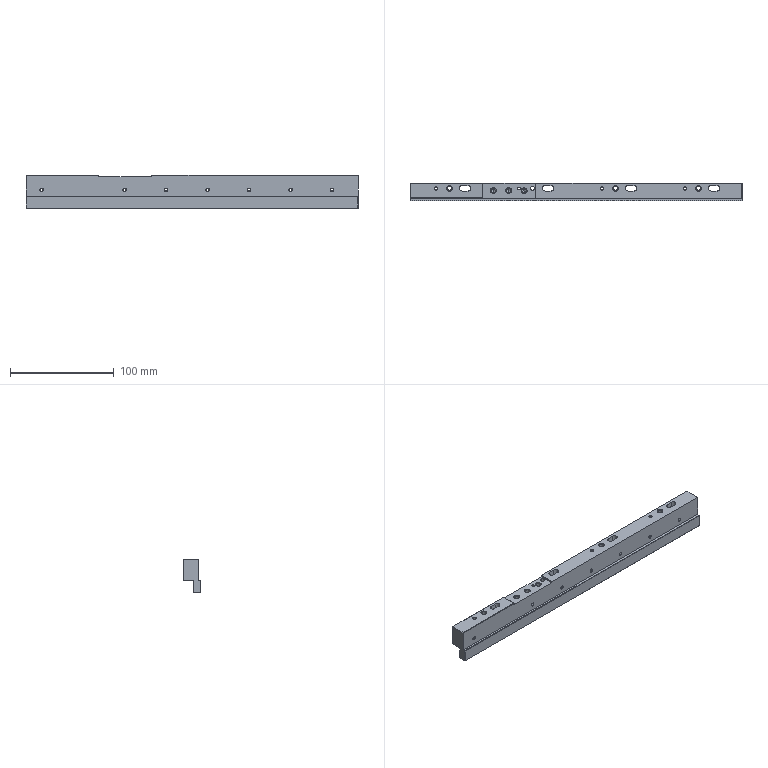Part | NX | 1 solid | 138 faces | box 320 x 17 x 32 mm | volume 111895 mm3 | cylinder 62 | plane 38 | cone 38 | commonest cylinder face diameters 2.5 x30 4.2 x20 5.2 x12